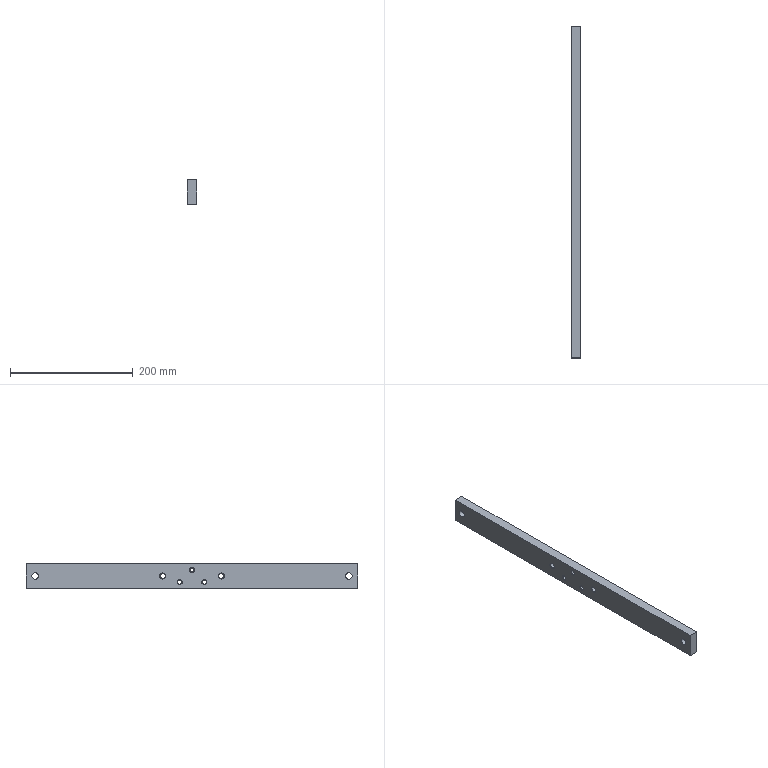Part | STEP file | 冲床-300配套压波_id1014_x_t | 1 solid | 23 faces | box 15 x 540 x 40 mm | volume 317910 mm3 | cone 10 | cylinder 7 | plane 6 | commonest cylinder face diameters 6.8 x3 8.5 x2 10.7 x2
STEP:
#1=CARTESIAN_POINT('',(1935.,-270.,-325.));
#2=VERTEX_POINT('',#1);
#3=CARTESIAN_POINT('',(1935.,-270.,-365.));
#4=VERTEX_POINT('',#3);
#5=CARTESIAN_POINT('',(1935.,-270.,-325.));
#6=DIRECTION('',(0.,0.,-1.));
#7=VECTOR('',#6,1.);
#8=LINE('',#5,#7);
#9=EDGE_CURVE('',#2,#4,#8,.T.);
#10=ORIENTED_EDGE('',*,*,#9,.F.);
#11=CARTESIAN_POINT('',(1920.,-270.,-325.));
#12=VERTEX_POINT('',#11);
#13=CARTESIAN_POINT('',(1920.,-270.,-325.));
#14=DIRECTION('',(1.,0.,0.));
#15=VECTOR('',#14,1.);
#16=LINE('',#13,#15);
#17=EDGE_CURVE('',#12,#2,#16,.T.);
#18=ORIENTED_EDGE('',*,*,#17,.F.);
#19=CARTESIAN_POINT('',(1920.,-270.,-365.));
#20=VERTEX_POINT('',#19);
#21=CARTESIAN_POINT('',(1920.,-270.,-325.));
#22=DIRECTION('',(0.,0.,-1.));
#23=VECTOR('',#22,1.);
#24=LINE('',#21,#23);
#25=EDGE_CURVE('',#12,#20,#24,.T.);
#26=ORIENTED_EDGE('',*,*,#25,.T.);
#27=CARTESIAN_POINT('',(1920.,-270.,-365.));
#28=DIRECTION('',(1.,0.,0.));
#29=VECTOR('',#28,1.);
#30=LINE('',#27,#29);
#31=EDGE_CURVE('',#20,#4,#30,.T.);
#32=ORIENTED_EDGE('',*,*,#31,.T.);
#33=EDGE_LOOP('',(#10,#18,#26,#32));
#34=FACE_OUTER_BOUND('',#33,.T.);
#35=CARTESIAN_POINT('',(1920.,-270.,-325.));
#36=DIRECTION('',(0.,-1.,0.));
#37=DIRECTION('',(0.,0.,-1.));
#38=AXIS2_PLACEMENT_3D('',#35,#36,#37);
#39=PLANE('',#38);
#40=ADVANCED_FACE('',(#34),#39,.T.);
#41=CARTESIAN_POINT('',(1935.,270.,-365.));
#42=VERTEX_POINT('',#41);
#43=CARTESIAN_POINT('',(1935.,-270.,-365.));
#44=DIRECTION('',(0.,1.,0.));
#45=VECTOR('',#44,1.);
#46=LINE('',#43,#45);
#47=EDGE_CURVE('',#4,#42,#46,.T.);
#48=ORIENTED_EDGE('',*,*,#47,.F.);
#49=ORIENTED_EDGE('',*,*,#31,.F.);
#50=CARTESIAN_POINT('',(1920.,270.,-365.));
#51=VERTEX_POINT('',#50);
#52=CARTESIAN_POINT('',(1920.,-270.,-365.));
#53=DIRECTION('',(0.,1.,0.));
#54=VECTOR('',#53,1.);
#55=LINE('',#52,#54);
#56=EDGE_CURVE('',#20,#51,#55,.T.);
#57=ORIENTED_EDGE('',*,*,#56,.T.);
#58=CARTESIAN_POINT('',(1920.,270.,-365.));
#59=DIRECTION('',(1.,0.,0.));
#60=VECTOR('',#59,1.);
#61=LINE('',#58,#60);
#62=EDGE_CURVE('',#51,#42,#61,.T.);
#63=ORIENTED_EDGE('',*,*,#62,.T.);
#64=EDGE_LOOP('',(#48,#49,#57,#63));
#65=FACE_OUTER_BOUND('',#64,.T.);
#66=CARTESIAN_POINT('',(1920.,-270.,-365.));
#67=DIRECTION('',(0.,0.,-1.));
#68=DIRECTION('',(0.,1.,0.));
#69=AXIS2_PLACEMENT_3D('',#66,#67,#68);
#70=PLANE('',#69);
#71=ADVANCED_FACE('',(#65),#70,.T.);
#72=CARTESIAN_POINT('',(1935.,270.,-325.));
#73=VERTEX_POINT('',#72);
#74=CARTESIAN_POINT('',(1935.,270.,-365.));
#75=DIRECTION('',(0.,0.,1.));
#76=VECTOR('',#75,1.);
#77=LINE('',#74,#76);
#78=EDGE_CURVE('',#42,#73,#77,.T.);
#79=ORIENTED_EDGE('',*,*,#78,.F.);
#80=ORIENTED_EDGE('',*,*,#62,.F.);
#81=CARTESIAN_POINT('',(1920.,270.,-325.));
#82=VERTEX_POINT('',#81);
#83=CARTESIAN_POINT('',(1920.,270.,-365.));
#84=DIRECTION('',(0.,0.,1.));
#85=VECTOR('',#84,1.);
#86=LINE('',#83,#85);
#87=EDGE_CURVE('',#51,#82,#86,.T.);
#88=ORIENTED_EDGE('',*,*,#87,.T.);
#89=CARTESIAN_POINT('',(1920.,270.,-325.));
#90=DIRECTION('',(1.,0.,0.));
#91=VECTOR('',#90,1.);
#92=LINE('',#89,#91);
#93=EDGE_CURVE('',#82,#73,#92,.T.);
#94=ORIENTED_EDGE('',*,*,#93,.T.);
#95=EDGE_LOOP('',(#79,#80,#88,#94));
#96=FACE_OUTER_BOUND('',#95,.T.);
#97=CARTESIAN_POINT('',(1920.,270.,-365.));
#98=DIRECTION('',(0.,1.,0.));
#99=DIRECTION('',(0.,0.,1.));
#100=AXIS2_PLACEMENT_3D('',#97,#98,#99);
#101=PLANE('',#100);
#102=ADVANCED_FACE('',(#96),#101,.T.);
#103=CARTESIAN_POINT('',(1935.,270.,-325.));
#104=DIRECTION('',(0.,-1.,0.));
#105=VECTOR('',#104,1.);
#106=LINE('',#103,#105);
#107=EDGE_CURVE('',#73,#2,#106,.T.);
#108=ORIENTED_EDGE('',*,*,#107,.F.);
#109=ORIENTED_EDGE('',*,*,#93,.F.);
#110=CARTESIAN_POINT('',(1920.,270.,-325.));
#111=DIRECTION('',(0.,-1.,0.));
#112=VECTOR('',#111,1.);
#113=LINE('',#110,#112);
#114=EDGE_CURVE('',#82,#12,#113,.T.);
#115=ORIENTED_EDGE('',*,*,#114,.T.);
#116=ORIENTED_EDGE('',*,*,#17,.T.);
#117=EDGE_LOOP('',(#108,#109,#115,#116));
#118=FACE_OUTER_BOUND('',#117,.T.);
#119=CARTESIAN_POINT('',(1920.,270.,-325.));
#120=DIRECTION('',(0.,0.,1.));
#121=DIRECTION('',(0.,-1.,0.));
#122=AXIS2_PLACEMENT_3D('',#119,#120,#121);
#123=PLANE('',#122);
#124=ADVANCED_FACE('',(#118),#123,.T.);
#125=CARTESIAN_POINT('',(1920.,-255.,-350.35));
#126=VERTEX_POINT('',#125);
#127=CARTESIAN_POINT('',(1920.,-255.,-345.));
#128=DIRECTION('',(-1.,0.,0.));
#129=DIRECTION('',(0.,0.,-1.));
#130=AXIS2_PLACEMENT_3D('',#127,#128,#129);
#131=CIRCLE('',#130,5.35);
#132=EDGE_CURVE('',#126,#126,#131,.T.);
#133=ORIENTED_EDGE('',*,*,#132,.F.);
#134=EDGE_LOOP('',(#133));
#135=FACE_BOUND('',#134,.T.);
#136=CARTESIAN_POINT('',(1920.,255.,-350.35));
#137=VERTEX_POINT('',#136);
#138=CARTESIAN_POINT('',(1920.,255.,-345.));
#139=DIRECTION('',(-1.,0.,0.));
#140=DIRECTION('',(0.,0.,-1.));
#141=AXIS2_PLACEMENT_3D('',#138,#139,#140);
#142=CIRCLE('',#141,5.35);
#143=EDGE_CURVE('',#137,#137,#142,.T.);
#144=ORIENTED_EDGE('',*,*,#143,.F.);
#145=EDGE_LOOP('',(#144));
#146=FACE_BOUND('',#145,.T.);
#147=CARTESIAN_POINT('',(1920.,47.5,-350.));
#148=VERTEX_POINT('',#147);
#149=CARTESIAN_POINT('',(1920.,47.5,-345.));
#150=DIRECTION('',(1.,0.,0.));
#151=DIRECTION('',(0.,0.,-1.));
#152=AXIS2_PLACEMENT_3D('',#149,#150,#151);
#153=CIRCLE('',#152,5.);
#154=EDGE_CURVE('',#148,#148,#153,.T.);
#155=ORIENTED_EDGE('',*,*,#154,.T.);
#156=EDGE_LOOP('',(#155));
#157=FACE_BOUND('',#156,.T.);
#158=CARTESIAN_POINT('',(1920.,-47.5,-350.));
#159=VERTEX_POINT('',#158);
#160=CARTESIAN_POINT('',(1920.,-47.5,-345.));
#161=DIRECTION('',(1.,0.,0.));
#162=DIRECTION('',(0.,0.,-1.));
#163=AXIS2_PLACEMENT_3D('',#160,#161,#162);
#164=CIRCLE('',#163,5.);
#165=EDGE_CURVE('',#159,#159,#164,.T.);
#166=ORIENTED_EDGE('',*,*,#165,.T.);
#167=EDGE_LOOP('',(#166));
#168=FACE_BOUND('',#167,.T.);
#169=CARTESIAN_POINT('',(1920.,0.,-339.));
#170=VERTEX_POINT('',#169);
#171=CARTESIAN_POINT('',(1920.,0.,-335.));
#172=DIRECTION('',(1.,0.,0.));
#173=DIRECTION('',(0.,0.,-1.));
#174=AXIS2_PLACEMENT_3D('',#171,#172,#173);
#175=CIRCLE('',#174,4.);
#176=EDGE_CURVE('',#170,#170,#175,.T.);
#177=ORIENTED_EDGE('',*,*,#176,.T.);
#178=EDGE_LOOP('',(#177));
#179=FACE_BOUND('',#178,.T.);
#180=CARTESIAN_POINT('',(1920.,20.,-359.));
#181=VERTEX_POINT('',#180);
#182=CARTESIAN_POINT('',(1920.,20.,-355.));
#183=DIRECTION('',(1.,0.,0.));
#184=DIRECTION('',(0.,0.,-1.));
#185=AXIS2_PLACEMENT_3D('',#182,#183,#184);
#186=CIRCLE('',#185,4.);
#187=EDGE_CURVE('',#181,#181,#186,.T.);
#188=ORIENTED_EDGE('',*,*,#187,.T.);
#189=EDGE_LOOP('',(#188));
#190=FACE_BOUND('',#189,.T.);
#191=CARTESIAN_POINT('',(1920.,-20.,-359.));
#192=VERTEX_POINT('',#191);
#193=CARTESIAN_POINT('',(1920.,-20.,-355.));
#194=DIRECTION('',(1.,0.,0.));
#195=DIRECTION('',(0.,0.,-1.));
#196=AXIS2_PLACEMENT_3D('',#193,#194,#195);
#197=CIRCLE('',#196,4.);
#198=EDGE_CURVE('',#192,#192,#197,.T.);
#199=ORIENTED_EDGE('',*,*,#198,.T.);
#200=EDGE_LOOP('',(#199));
#201=FACE_BOUND('',#200,.T.);
#202=ORIENTED_EDGE('',*,*,#25,.F.);
#203=ORIENTED_EDGE('',*,*,#114,.F.);
#204=ORIENTED_EDGE('',*,*,#87,.F.);
#205=ORIENTED_EDGE('',*,*,#56,.F.);
#206=EDGE_LOOP('',(#202,#203,#204,#205));
#207=FACE_BOUND('',#206,.T.);
#208=CARTESIAN_POINT('',(1920.,0.,-125.));
#209=DIRECTION('',(1.,0.,0.));
#210=DIRECTION('',(0.,0.,-1.));
#211=AXIS2_PLACEMENT_3D('',#208,#209,#210);
#212=PLANE('',#211);
#213=ADVANCED_FACE('',(#135,#146,#157,#168,#179,#190,#201,#207),#212,.F.);
#214=CARTESIAN_POINT('',(1935.,-255.,-350.35));
#215=VERTEX_POINT('',#214);
#216=CARTESIAN_POINT('',(1935.,-255.,-345.));
#217=DIRECTION('',(-1.,0.,0.));
#218=DIRECTION('',(0.,0.,-1.));
#219=AXIS2_PLACEMENT_3D('',#216,#217,#218);
#220=CIRCLE('',#219,5.35);
#221=EDGE_CURVE('',#215,#215,#220,.T.);
#222=ORIENTED_EDGE('',*,*,#221,.T.);
#223=EDGE_LOOP('',(#222));
#224=FACE_BOUND('',#223,.T.);
#225=CARTESIAN_POINT('',(1935.,255.,-350.35));
#226=VERTEX_POINT('',#225);
#227=CARTESIAN_POINT('',(1935.,255.,-345.));
#228=DIRECTION('',(-1.,0.,0.));
#229=DIRECTION('',(0.,0.,-1.));
#230=AXIS2_PLACEMENT_3D('',#227,#228,#229);
#231=CIRCLE('',#230,5.35);
#232=EDGE_CURVE('',#226,#226,#231,.T.);
#233=ORIENTED_EDGE('',*,*,#232,.T.);
#234=EDGE_LOOP('',(#233));
#235=FACE_BOUND('',#234,.T.);
#236=CARTESIAN_POINT('',(1935.,47.5,-350.));
#237=VERTEX_POINT('',#236);
#238=CARTESIAN_POINT('',(1935.,47.5,-345.));
#239=DIRECTION('',(-1.,0.,0.));
#240=DIRECTION('',(0.,0.,-1.));
#241=AXIS2_PLACEMENT_3D('',#238,#239,#240);
#242=CIRCLE('',#241,5.);
#243=EDGE_CURVE('',#237,#237,#242,.T.);
#244=ORIENTED_EDGE('',*,*,#243,.T.);
#245=EDGE_LOOP('',(#244));
#246=FACE_BOUND('',#245,.T.);
#247=CARTESIAN_POINT('',(1935.,-47.5,-350.));
#248=VERTEX_POINT('',#247);
#249=CARTESIAN_POINT('',(1935.,-47.5,-345.));
#250=DIRECTION('',(-1.,0.,0.));
#251=DIRECTION('',(0.,0.,-1.));
#252=AXIS2_PLACEMENT_3D('',#249,#250,#251);
#253=CIRCLE('',#252,5.);
#254=EDGE_CURVE('',#248,#248,#253,.T.);
#255=ORIENTED_EDGE('',*,*,#254,.T.);
#256=EDGE_LOOP('',(#255));
#257=FACE_BOUND('',#256,.T.);
#258=CARTESIAN_POINT('',(1935.,0.,-339.));
#259=VERTEX_POINT('',#258);
#260=CARTESIAN_POINT('',(1935.,0.,-335.));
#261=DIRECTION('',(-1.,0.,0.));
#262=DIRECTION('',(0.,0.,-1.));
#263=AXIS2_PLACEMENT_3D('',#260,#261,#262);
#264=CIRCLE('',#263,4.);
#265=EDGE_CURVE('',#259,#259,#264,.T.);
#266=ORIENTED_EDGE('',*,*,#265,.T.);
#267=EDGE_LOOP('',(#266));
#268=FACE_BOUND('',#267,.T.);
#269=CARTESIAN_POINT('',(1935.,20.,-359.));
#270=VERTEX_POINT('',#269);
#271=CARTESIAN_POINT('',(1935.,20.,-355.));
#272=DIRECTION('',(-1.,0.,0.));
#273=DIRECTION('',(0.,0.,-1.));
#274=AXIS2_PLACEMENT_3D('',#271,#272,#273);
#275=CIRCLE('',#274,4.);
#276=EDGE_CURVE('',#270,#270,#275,.T.);
#277=ORIENTED_EDGE('',*,*,#276,.T.);
#278=EDGE_LOOP('',(#277));
#279=FACE_BOUND('',#278,.T.);
#280=CARTESIAN_POINT('',(1935.,-20.,-359.));
#281=VERTEX_POINT('',#280);
#282=CARTESIAN_POINT('',(1935.,-20.,-355.));
#283=DIRECTION('',(-1.,0.,0.));
#284=DIRECTION('',(0.,0.,-1.));
#285=AXIS2_PLACEMENT_3D('',#282,#283,#284);
#286=CIRCLE('',#285,4.);
#287=EDGE_CURVE('',#281,#281,#286,.T.);
#288=ORIENTED_EDGE('',*,*,#287,.T.);
#289=EDGE_LOOP('',(#288));
#290=FACE_BOUND('',#289,.T.);
#291=ORIENTED_EDGE('',*,*,#9,.T.);
#292=ORIENTED_EDGE('',*,*,#47,.T.);
#293=ORIENTED_EDGE('',*,*,#78,.T.);
#294=ORIENTED_EDGE('',*,*,#107,.T.);
#295=EDGE_LOOP('',(#291,#292,#293,#294));
#296=FACE_BOUND('',#295,.T.);
#297=CARTESIAN_POINT('',(1935.,0.,-125.));
#298=DIRECTION('',(1.,0.,0.));
#299=DIRECTION('',(0.,0.,-1.));
#300=AXIS2_PLACEMENT_3D('',#297,#298,#299);
#301=PLANE('',#300);
#302=ADVANCED_FACE('',(#224,#235,#246,#257,#268,#279,#290,#296),#301,.T.);
#303=CARTESIAN_POINT('',(1920.6,-20.,-358.4));
#304=VERTEX_POINT('',#303);
#305=CARTESIAN_POINT('',(1920.6,-20.,-355.));
#306=DIRECTION('',(-1.,0.,0.));
#307=DIRECTION('',(0.,0.,-1.));
#308=AXIS2_PLACEMENT_3D('',#305,#306,#307);
#309=CIRCLE('',#308,3.4);
#310=EDGE_CURVE('',#304,#304,#309,.T.);
#311=ORIENTED_EDGE('',*,*,#310,.T.);
#312=EDGE_LOOP('',(#311));
#313=FACE_BOUND('',#312,.T.);
#314=CARTESIAN_POINT('',(1934.4,-20.,-358.4));
#315=VERTEX_POINT('',#314);
#316=CARTESIAN_POINT('',(1934.4,-20.,-355.));
#317=DIRECTION('',(1.,0.,0.));
#318=DIRECTION('',(0.,0.,-1.));
#319=AXIS2_PLACEMENT_3D('',#316,#317,#318);
#320=CIRCLE('',#319,3.4);
#321=EDGE_CURVE('',#315,#315,#320,.T.);
#322=ORIENTED_EDGE('',*,*,#321,.T.);
#323=EDGE_LOOP('',(#322));
#324=FACE_BOUND('',#323,.T.);
#325=CARTESIAN_POINT('',(1935.,-20.,-355.));
#326=DIRECTION('',(-1.,0.,0.));
#327=DIRECTION('',(0.,0.,1.));
#328=AXIS2_PLACEMENT_3D('',#325,#326,#327);
#329=CYLINDRICAL_SURFACE('',#328,3.4);
#330=ADVANCED_FACE('',(#313,#324),#329,.F.);
#331=ORIENTED_EDGE('',*,*,#321,.F.);
#332=EDGE_LOOP('',(#331));
#333=FACE_BOUND('',#332,.T.);
#334=ORIENTED_EDGE('',*,*,#287,.F.);
#335=EDGE_LOOP('',(#334));
#336=FACE_BOUND('',#335,.T.);
#337=CARTESIAN_POINT('',(1935.,-20.,-355.));
#338=DIRECTION('',(1.,0.,0.));
#339=DIRECTION('',(0.,0.,-1.));
#340=AXIS2_PLACEMENT_3D('',#337,#338,#339);
#341=CONICAL_SURFACE('',#340,4.,45.);
#342=ADVANCED_FACE('',(#333,#336),#341,.F.);
#343=ORIENTED_EDGE('',*,*,#310,.F.);
#344=EDGE_LOOP('',(#343));
#345=FACE_BOUND('',#344,.T.);
#346=ORIENTED_EDGE('',*,*,#198,.F.);
#347=EDGE_LOOP('',(#346));
#348=FACE_BOUND('',#347,.T.);
#349=CARTESIAN_POINT('',(1920.,-20.,-355.));
#350=DIRECTION('',(-1.,0.,0.));
#351=DIRECTION('',(0.,0.,1.));
#352=AXIS2_PLACEMENT_3D('',#349,#350,#351);
#353=CONICAL_SURFACE('',#352,4.,45.);
#354=ADVANCED_FACE('',(#345,#348),#353,.F.);
#355=CARTESIAN_POINT('',(1920.6,20.,-358.4));
#356=VERTEX_POINT('',#355);
#357=CARTESIAN_POINT('',(1920.6,20.,-355.));
#358=DIRECTION('',(-1.,0.,0.));
#359=DIRECTION('',(0.,0.,-1.));
#360=AXIS2_PLACEMENT_3D('',#357,#358,#359);
#361=CIRCLE('',#360,3.4);
#362=EDGE_CURVE('',#356,#356,#361,.T.);
#363=ORIENTED_EDGE('',*,*,#362,.T.);
#364=EDGE_LOOP('',(#363));
#365=FACE_BOUND('',#364,.T.);
#366=CARTESIAN_POINT('',(1934.4,20.,-358.4));
#367=VERTEX_POINT('',#366);
#368=CARTESIAN_POINT('',(1934.4,20.,-355.));
#369=DIRECTION('',(1.,0.,0.));
#370=DIRECTION('',(0.,0.,-1.));
#371=AXIS2_PLACEMENT_3D('',#368,#369,#370);
#372=CIRCLE('',#371,3.4);
#373=EDGE_CURVE('',#367,#367,#372,.T.);
#374=ORIENTED_EDGE('',*,*,#373,.T.);
#375=EDGE_LOOP('',(#374));
#376=FACE_BOUND('',#375,.T.);
#377=CARTESIAN_POINT('',(1935.,20.,-355.));
#378=DIRECTION('',(-1.,0.,0.));
#379=DIRECTION('',(0.,0.,1.));
#380=AXIS2_PLACEMENT_3D('',#377,#378,#379);
#381=CYLINDRICAL_SURFACE('',#380,3.4);
#382=ADVANCED_FACE('',(#365,#376),#381,.F.);
#383=ORIENTED_EDGE('',*,*,#373,.F.);
#384=EDGE_LOOP('',(#383));
#385=FACE_BOUND('',#384,.T.);
#386=ORIENTED_EDGE('',*,*,#276,.F.);
#387=EDGE_LOOP('',(#386));
#388=FACE_BOUND('',#387,.T.);
#389=CARTESIAN_POINT('',(1935.,20.,-355.));
#390=DIRECTION('',(1.,0.,0.));
#391=DIRECTION('',(0.,0.,-1.));
#392=AXIS2_PLACEMENT_3D('',#389,#390,#391);
#393=CONICAL_SURFACE('',#392,4.,45.);
#394=ADVANCED_FACE('',(#385,#388),#393,.F.);
#395=ORIENTED_EDGE('',*,*,#362,.F.);
#396=EDGE_LOOP('',(#395));
#397=FACE_BOUND('',#396,.T.);
#398=ORIENTED_EDGE('',*,*,#187,.F.);
#399=EDGE_LOOP('',(#398));
#400=FACE_BOUND('',#399,.T.);
#401=CARTESIAN_POINT('',(1920.,20.,-355.));
#402=DIRECTION('',(-1.,0.,0.));
#403=DIRECTION('',(0.,0.,1.));
#404=AXIS2_PLACEMENT_3D('',#401,#402,#403);
#405=CONICAL_SURFACE('',#404,4.,45.);
#406=ADVANCED_FACE('',(#397,#400),#405,.F.);
#407=CARTESIAN_POINT('',(1920.6,0.,-338.4));
#408=VERTEX_POINT('',#407);
#409=CARTESIAN_POINT('',(1920.6,0.,-335.));
#410=DIRECTION('',(-1.,0.,0.));
#411=DIRECTION('',(0.,0.,-1.));
#412=AXIS2_PLACEMENT_3D('',#409,#410,#411);
#413=CIRCLE('',#412,3.4);
#414=EDGE_CURVE('',#408,#408,#413,.T.);
#415=ORIENTED_EDGE('',*,*,#414,.T.);
#416=EDGE_LOOP('',(#415));
#417=FACE_BOUND('',#416,.T.);
#418=CARTESIAN_POINT('',(1934.4,0.,-338.4));
#419=VERTEX_POINT('',#418);
#420=CARTESIAN_POINT('',(1934.4,0.,-335.));
#421=DIRECTION('',(1.,0.,0.));
#422=DIRECTION('',(0.,0.,-1.));
#423=AXIS2_PLACEMENT_3D('',#420,#421,#422);
#424=CIRCLE('',#423,3.4);
#425=EDGE_CURVE('',#419,#419,#424,.T.);
#426=ORIENTED_EDGE('',*,*,#425,.T.);
#427=EDGE_LOOP('',(#426));
#428=FACE_BOUND('',#427,.T.);
#429=CARTESIAN_POINT('',(1935.,0.,-335.));
#430=DIRECTION('',(-1.,0.,0.));
#431=DIRECTION('',(0.,0.,1.));
#432=AXIS2_PLACEMENT_3D('',#429,#430,#431);
#433=CYLINDRICAL_SURFACE('',#432,3.4);
#434=ADVANCED_FACE('',(#417,#428),#433,.F.);
#435=ORIENTED_EDGE('',*,*,#425,.F.);
#436=EDGE_LOOP('',(#435));
#437=FACE_BOUND('',#436,.T.);
#438=ORIENTED_EDGE('',*,*,#265,.F.);
#439=EDGE_LOOP('',(#438));
#440=FACE_BOUND('',#439,.T.);
#441=CARTESIAN_POINT('',(1935.,0.,-335.));
#442=DIRECTION('',(1.,0.,0.));
#443=DIRECTION('',(0.,0.,-1.));
#444=AXIS2_PLACEMENT_3D('',#441,#442,#443);
#445=CONICAL_SURFACE('',#444,4.,45.);
#446=ADVANCED_FACE('',(#437,#440),#445,.F.);
#447=ORIENTED_EDGE('',*,*,#414,.F.);
#448=EDGE_LOOP('',(#447));
#449=FACE_BOUND('',#448,.T.);
#450=ORIENTED_EDGE('',*,*,#176,.F.);
#451=EDGE_LOOP('',(#450));
#452=FACE_BOUND('',#451,.T.);
#453=CARTESIAN_POINT('',(1920.,0.,-335.));
#454=DIRECTION('',(-1.,0.,0.));
#455=DIRECTION('',(0.,0.,1.));
#456=AXIS2_PLACEMENT_3D('',#453,#454,#455);
#457=CONICAL_SURFACE('',#456,4.,45.);
#458=ADVANCED_FACE('',(#449,#452),#457,.F.);
#459=CARTESIAN_POINT('',(1920.75,-47.5,-349.25));
#460=VERTEX_POINT('',#459);
#461=CARTESIAN_POINT('',(1920.75,-47.5,-345.));
#462=DIRECTION('',(-1.,0.,0.));
#463=DIRECTION('',(0.,0.,-1.));
#464=AXIS2_PLACEMENT_3D('',#461,#462,#463);
#465=CIRCLE('',#464,4.25);
#466=EDGE_CURVE('',#460,#460,#465,.T.);
#467=ORIENTED_EDGE('',*,*,#466,.T.);
#468=EDGE_LOOP('',(#467));
#469=FACE_BOUND('',#468,.T.);
#470=CARTESIAN_POINT('',(1934.25,-47.5,-349.25));
#471=VERTEX_POINT('',#470);
#472=CARTESIAN_POINT('',(1934.25,-47.5,-345.));
#473=DIRECTION('',(1.,0.,0.));
#474=DIRECTION('',(0.,0.,-1.));
#475=AXIS2_PLACEMENT_3D('',#472,#473,#474);
#476=CIRCLE('',#475,4.25);
#477=EDGE_CURVE('',#471,#471,#476,.T.);
#478=ORIENTED_EDGE('',*,*,#477,.T.);
#479=EDGE_LOOP('',(#478));
#480=FACE_BOUND('',#479,.T.);
#481=CARTESIAN_POINT('',(1935.,-47.5,-345.));
#482=DIRECTION('',(-1.,0.,0.));
#483=DIRECTION('',(0.,0.,1.));
#484=AXIS2_PLACEMENT_3D('',#481,#482,#483);
#485=CYLINDRICAL_SURFACE('',#484,4.25);
#486=ADVANCED_FACE('',(#469,#480),#485,.F.);
#487=ORIENTED_EDGE('',*,*,#477,.F.);
#488=EDGE_LOOP('',(#487));
#489=FACE_BOUND('',#488,.T.);
#490=ORIENTED_EDGE('',*,*,#254,.F.);
#491=EDGE_LOOP('',(#490));
#492=FACE_BOUND('',#491,.T.);
#493=CARTESIAN_POINT('',(1935.,-47.5,-345.));
#494=DIRECTION('',(1.,0.,0.));
#495=DIRECTION('',(0.,0.,-1.));
#496=AXIS2_PLACEMENT_3D('',#493,#494,#495);
#497=CONICAL_SURFACE('',#496,5.,45.);
#498=ADVANCED_FACE('',(#489,#492),#497,.F.);
#499=ORIENTED_EDGE('',*,*,#466,.F.);
#500=EDGE_LOOP('',(#499));
#501=FACE_BOUND('',#500,.T.);
#502=ORIENTED_EDGE('',*,*,#165,.F.);
#503=EDGE_LOOP('',(#502));
#504=FACE_BOUND('',#503,.T.);
#505=CARTESIAN_POINT('',(1920.,-47.5,-345.));
#506=DIRECTION('',(-1.,0.,0.));
#507=DIRECTION('',(0.,0.,1.));
#508=AXIS2_PLACEMENT_3D('',#505,#506,#507);
#509=CONICAL_SURFACE('',#508,5.,45.);
#510=ADVANCED_FACE('',(#501,#504),#509,.F.);
#511=CARTESIAN_POINT('',(1920.75,47.5,-349.25));
#512=VERTEX_POINT('',#511);
#513=CARTESIAN_POINT('',(1920.75,47.5,-345.));
#514=DIRECTION('',(-1.,0.,0.));
#515=DIRECTION('',(0.,0.,-1.));
#516=AXIS2_PLACEMENT_3D('',#513,#514,#515);
#517=CIRCLE('',#516,4.25);
#518=EDGE_CURVE('',#512,#512,#517,.T.);
#519=ORIENTED_EDGE('',*,*,#518,.T.);
#520=EDGE_LOOP('',(#519));
#521=FACE_BOUND('',#520,.T.);
#522=CARTESIAN_POINT('',(1934.25,47.5,-349.25));
#523=VERTEX_POINT('',#522);
#524=CARTESIAN_POINT('',(1934.25,47.5,-345.));
#525=DIRECTION('',(1.,0.,0.));
#526=DIRECTION('',(0.,0.,-1.));
#527=AXIS2_PLACEMENT_3D('',#524,#525,#526);
#528=CIRCLE('',#527,4.25);
#529=EDGE_CURVE('',#523,#523,#528,.T.);
#530=ORIENTED_EDGE('',*,*,#529,.T.);
#531=EDGE_LOOP('',(#530));
#532=FACE_BOUND('',#531,.T.);
#533=CARTESIAN_POINT('',(1935.,47.5,-345.));
#534=DIRECTION('',(-1.,0.,0.));
#535=DIRECTION('',(0.,0.,1.));
#536=AXIS2_PLACEMENT_3D('',#533,#534,#535);
#537=CYLINDRICAL_SURFACE('',#536,4.25);
#538=ADVANCED_FACE('',(#521,#532),#537,.F.);
#539=ORIENTED_EDGE('',*,*,#529,.F.);
#540=EDGE_LOOP('',(#539));
#541=FACE_BOUND('',#540,.T.);
#542=ORIENTED_EDGE('',*,*,#243,.F.);
#543=EDGE_LOOP('',(#542));
#544=FACE_BOUND('',#543,.T.);
#545=CARTESIAN_POINT('',(1935.,47.5,-345.));
#546=DIRECTION('',(1.,0.,0.));
#547=DIRECTION('',(0.,0.,-1.));
#548=AXIS2_PLACEMENT_3D('',#545,#546,#547);
#549=CONICAL_SURFACE('',#548,5.,45.);
#550=ADVANCED_FACE('',(#541,#544),#549,.F.);
#551=ORIENTED_EDGE('',*,*,#518,.F.);
#552=EDGE_LOOP('',(#551));
#553=FACE_BOUND('',#552,.T.);
#554=ORIENTED_EDGE('',*,*,#154,.F.);
#555=EDGE_LOOP('',(#554));
#556=FACE_BOUND('',#555,.T.);
#557=CARTESIAN_POINT('',(1920.,47.5,-345.));
#558=DIRECTION('',(-1.,0.,0.));
#559=DIRECTION('',(0.,0.,1.));
#560=AXIS2_PLACEMENT_3D('',#557,#558,#559);
#561=CONICAL_SURFACE('',#560,5.,45.);
#562=ADVANCED_FACE('',(#553,#556),#561,.F.);
#563=ORIENTED_EDGE('',*,*,#232,.F.);
#564=EDGE_LOOP('',(#563));
#565=FACE_BOUND('',#564,.T.);
#566=ORIENTED_EDGE('',*,*,#143,.T.);
#567=EDGE_LOOP('',(#566));
#568=FACE_BOUND('',#567,.T.);
#569=CARTESIAN_POINT('',(2085.,255.,-345.));
#570=DIRECTION('',(-1.,0.,0.));
#571=DIRECTION('',(0.,0.,1.));
#572=AXIS2_PLACEMENT_3D('',#569,#570,#571);
#573=CYLINDRICAL_SURFACE('',#572,5.35);
#574=ADVANCED_FACE('',(#565,#568),#573,.F.);
#575=ORIENTED_EDGE('',*,*,#221,.F.);
#576=EDGE_LOOP('',(#575));
#577=FACE_BOUND('',#576,.T.);
#578=ORIENTED_EDGE('',*,*,#132,.T.);
#579=EDGE_LOOP('',(#578));
#580=FACE_BOUND('',#579,.T.);
#581=CARTESIAN_POINT('',(2085.,-255.,-345.));
#582=DIRECTION('',(-1.,0.,0.));
#583=DIRECTION('',(0.,0.,1.));
#584=AXIS2_PLACEMENT_3D('',#581,#582,#583);
#585=CYLINDRICAL_SURFACE('',#584,5.35);
#586=ADVANCED_FACE('',(#577,#580),#585,.F.);
#587=CLOSED_SHELL('',(#40,#71,#102,#124,#213,#302,#330,#342,#354,#382,#394,#406,#434,#446,#458,#486,#498,#510,#538,#550,#562,#574,#586));
#588=MANIFOLD_SOLID_BREP('',#587);
#589=(LENGTH_UNIT()NAMED_UNIT(*)SI_UNIT(.MILLI.,.METRE.));
#590=UNCERTAINTY_MEASURE_WITH_UNIT(LENGTH_MEASURE(0.00002),#589,'','');
#591=(NAMED_UNIT(*)PLANE_ANGLE_UNIT()SI_UNIT($,.RADIAN.));
#592=PLANE_ANGLE_MEASURE_WITH_UNIT(PLANE_ANGLE_MEASURE(0.01745),#591);
#593=DIMENSIONAL_EXPONENTS(0.,0.,0.,0.,0.,0.,0.);
#594=(CONVERSION_BASED_UNIT('DEGREE',#592)NAMED_UNIT(#593)PLANE_ANGLE_UNIT());
#595=(NAMED_UNIT(*)SI_UNIT($,.STERADIAN.)SOLID_ANGLE_UNIT());
#596=(GEOMETRIC_REPRESENTATION_CONTEXT(3)GLOBAL_UNCERTAINTY_ASSIGNED_CONTEXT((#590))GLOBAL_UNIT_ASSIGNED_CONTEXT((#589,#594,#595))REPRESENTATION_CONTEXT('',''));
#597=ADVANCED_BREP_SHAPE_REPRESENTATION('',(#588),#596);